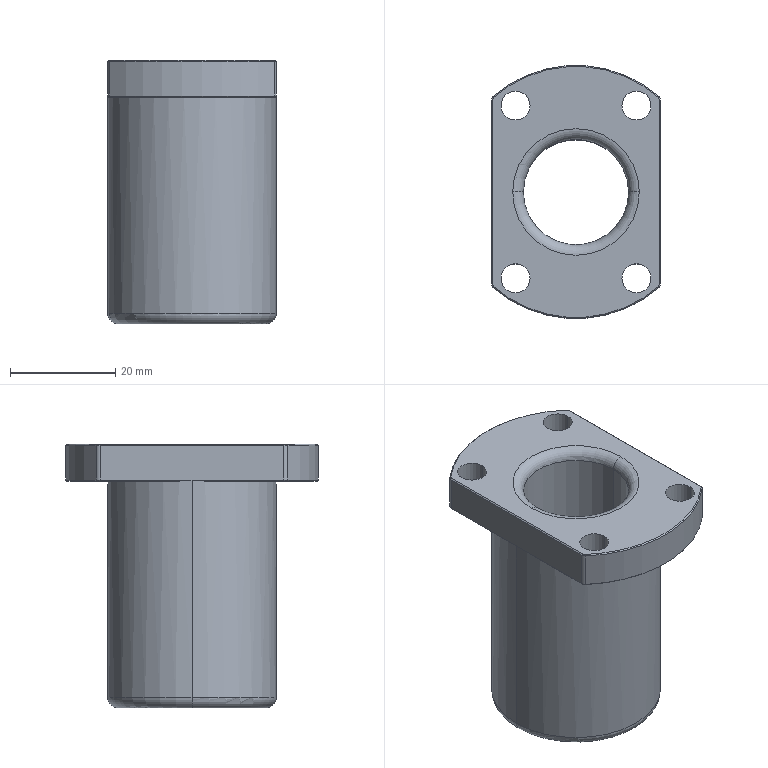Part | Creo | features DATUM PLANE 3, ROUND 3, CURVE 2, PROTRUSION 2, CHAMFER 1, COORDINATE SYSTEM 1 | 1 solid | 48 faces | box 32 x 48 x 50 mm | volume 27898 mm3 | cylinder 18 | plane 12 | cone 12 | torus 6 | commonest cylinder face diameters 5.5 x8 2 x4 20 x2 32 x2 48 x2
STEP:
#1=CARTESIAN_POINT('',(0.,0.,0.));
#2=DIRECTION('',(0.,0.,1.));
#3=DIRECTION('',(1.,0.,0.));
#4=AXIS2_PLACEMENT_3D('',#1,#2,#3);
#5=CARTESIAN_POINT('',(15.8,-2.522,0.));
#6=VERTEX_POINT('',#5);
#7=CARTESIAN_POINT('',(15.8,-17.436,-0.000000006));
#8=VERTEX_POINT('',#7);
#9=CARTESIAN_POINT('',(15.8,-2.522,0.));
#10=DIRECTION('',(0.,-1.,0.));
#11=VECTOR('',#10,14.914);
#12=LINE('',#9,#11);
#13=EDGE_CURVE('',#6,#8,#12,.T.);
#14=ORIENTED_EDGE('',*,*,#13,.F.);
#15=CARTESIAN_POINT('',(-15.8,-2.522,0.));
#16=VERTEX_POINT('',#15);
#17=CARTESIAN_POINT('',(0.,0.,0.));
#18=DIRECTION('',(0.,0.,-1.));
#19=DIRECTION('',(0.9875,-0.1576,0.));
#20=AXIS2_PLACEMENT_3D('',#17,#18,#19);
#21=CIRCLE('',#20,16.);
#22=EDGE_CURVE('',#6,#16,#21,.T.);
#23=ORIENTED_EDGE('',*,*,#22,.T.);
#24=CARTESIAN_POINT('',(-15.8,-17.436,0.));
#25=VERTEX_POINT('',#24);
#26=CARTESIAN_POINT('',(-15.8,-17.436,-0.000000002));
#27=DIRECTION('',(0.,1.,0.));
#28=VECTOR('',#27,14.914);
#29=LINE('',#26,#28);
#30=EDGE_CURVE('',#25,#16,#29,.T.);
#31=ORIENTED_EDGE('',*,*,#30,.F.);
#32=CARTESIAN_POINT('',(-15.522,-18.042,0.));
#33=VERTEX_POINT('',#32);
#34=CARTESIAN_POINT('',(-15.,-17.436,0.));
#35=DIRECTION('',(0.,0.,-1.));
#36=DIRECTION('',(-0.6522,-0.7581,0.));
#37=AXIS2_PLACEMENT_3D('',#34,#35,#36);
#38=CIRCLE('',#37,0.8);
#39=EDGE_CURVE('',#33,#25,#38,.T.);
#40=ORIENTED_EDGE('',*,*,#39,.F.);
#41=CARTESIAN_POINT('',(15.522,-18.042,0.));
#42=VERTEX_POINT('',#41);
#43=CARTESIAN_POINT('',(0.,0.,0.));
#44=DIRECTION('',(0.,0.,-1.));
#45=DIRECTION('',(0.6522,-0.7581,0.));
#46=AXIS2_PLACEMENT_3D('',#43,#44,#45);
#47=CIRCLE('',#46,23.8);
#48=EDGE_CURVE('',#42,#33,#47,.T.);
#49=ORIENTED_EDGE('',*,*,#48,.F.);
#50=CARTESIAN_POINT('',(15.,-17.436,0.));
#51=DIRECTION('',(0.,0.,-1.));
#52=DIRECTION('',(1.,0.,0.));
#53=AXIS2_PLACEMENT_3D('',#50,#51,#52);
#54=CIRCLE('',#53,0.8);
#55=EDGE_CURVE('',#8,#42,#54,.T.);
#56=ORIENTED_EDGE('',*,*,#55,.F.);
#57=EDGE_LOOP('',(#14,#23,#31,#40,#49,#56));
#58=FACE_OUTER_BOUND('',#57,.F.);
#59=CARTESIAN_POINT('',(14.222,-16.38,0.));
#60=VERTEX_POINT('',#59);
#61=CARTESIAN_POINT('',(8.722,-16.38,0.));
#62=VERTEX_POINT('',#61);
#63=CARTESIAN_POINT('',(11.472,-16.38,0.));
#64=DIRECTION('',(0.,0.,-1.));
#65=DIRECTION('',(1.,0.,0.));
#66=AXIS2_PLACEMENT_3D('',#63,#64,#65);
#67=CIRCLE('',#66,2.75);
#68=EDGE_CURVE('',#60,#62,#67,.T.);
#69=ORIENTED_EDGE('',*,*,#68,.T.);
#70=CARTESIAN_POINT('',(11.472,-16.38,0.));
#71=DIRECTION('',(0.,0.,-1.));
#72=DIRECTION('',(-1.,0.,0.));
#73=AXIS2_PLACEMENT_3D('',#70,#71,#72);
#74=CIRCLE('',#73,2.75);
#75=EDGE_CURVE('',#62,#60,#74,.T.);
#76=ORIENTED_EDGE('',*,*,#75,.T.);
#77=EDGE_LOOP('',(#69,#76));
#78=FACE_BOUND('',#77,.F.);
#79=CARTESIAN_POINT('',(-8.722,-16.38,0.));
#80=VERTEX_POINT('',#79);
#81=CARTESIAN_POINT('',(-14.222,-16.38,0.));
#82=VERTEX_POINT('',#81);
#83=CARTESIAN_POINT('',(-11.472,-16.38,0.));
#84=DIRECTION('',(0.,0.,-1.));
#85=DIRECTION('',(1.,0.,0.));
#86=AXIS2_PLACEMENT_3D('',#83,#84,#85);
#87=CIRCLE('',#86,2.75);
#88=EDGE_CURVE('',#80,#82,#87,.T.);
#89=ORIENTED_EDGE('',*,*,#88,.T.);
#90=CARTESIAN_POINT('',(-11.472,-16.38,0.));
#91=DIRECTION('',(0.,0.,-1.));
#92=DIRECTION('',(-1.,0.,0.));
#93=AXIS2_PLACEMENT_3D('',#90,#91,#92);
#94=CIRCLE('',#93,2.75);
#95=EDGE_CURVE('',#82,#80,#94,.T.);
#96=ORIENTED_EDGE('',*,*,#95,.T.);
#97=EDGE_LOOP('',(#89,#96));
#98=FACE_BOUND('',#97,.F.);
#99=CARTESIAN_POINT('',(0.,0.,0.));
#100=DIRECTION('',(0.,0.,1.));
#101=DIRECTION('',(1.,0.,0.));
#102=AXIS2_PLACEMENT_3D('',#99,#100,#101);
#103=PLANE('',#102);
#104=ADVANCED_FACE('',(#58,#78,#98),#103,.F.);
#105=CARTESIAN_POINT('',(15.8,17.436,-0.000000002));
#106=VERTEX_POINT('',#105);
#107=CARTESIAN_POINT('',(15.8,2.522,0.));
#108=VERTEX_POINT('',#107);
#109=CARTESIAN_POINT('',(15.8,17.436,-0.000000002));
#110=DIRECTION('',(0.,-1.,0.));
#111=VECTOR('',#110,14.914);
#112=LINE('',#109,#111);
#113=EDGE_CURVE('',#106,#108,#112,.T.);
#114=ORIENTED_EDGE('',*,*,#113,.F.);
#115=CARTESIAN_POINT('',(15.522,18.042,0.));
#116=VERTEX_POINT('',#115);
#117=CARTESIAN_POINT('',(15.,17.436,0.));
#118=DIRECTION('',(0.,0.,-1.));
#119=DIRECTION('',(0.6522,0.7581,0.));
#120=AXIS2_PLACEMENT_3D('',#117,#118,#119);
#121=CIRCLE('',#120,0.8);
#122=EDGE_CURVE('',#116,#106,#121,.T.);
#123=ORIENTED_EDGE('',*,*,#122,.F.);
#124=CARTESIAN_POINT('',(-15.522,18.042,0.));
#125=VERTEX_POINT('',#124);
#126=CARTESIAN_POINT('',(0.,0.,0.));
#127=DIRECTION('',(0.,0.,-1.));
#128=DIRECTION('',(-0.6522,0.7581,0.));
#129=AXIS2_PLACEMENT_3D('',#126,#127,#128);
#130=CIRCLE('',#129,23.8);
#131=EDGE_CURVE('',#125,#116,#130,.T.);
#132=ORIENTED_EDGE('',*,*,#131,.F.);
#133=CARTESIAN_POINT('',(-15.8,17.436,0.));
#134=VERTEX_POINT('',#133);
#135=CARTESIAN_POINT('',(-15.,17.436,0.));
#136=DIRECTION('',(0.,0.,-1.));
#137=DIRECTION('',(-1.,0.,0.));
#138=AXIS2_PLACEMENT_3D('',#135,#136,#137);
#139=CIRCLE('',#138,0.8);
#140=EDGE_CURVE('',#134,#125,#139,.T.);
#141=ORIENTED_EDGE('',*,*,#140,.F.);
#142=CARTESIAN_POINT('',(-15.8,2.522,0.));
#143=VERTEX_POINT('',#142);
#144=CARTESIAN_POINT('',(-15.8,2.522,0.));
#145=DIRECTION('',(0.,1.,0.));
#146=VECTOR('',#145,14.914);
#147=LINE('',#144,#146);
#148=EDGE_CURVE('',#143,#134,#147,.T.);
#149=ORIENTED_EDGE('',*,*,#148,.F.);
#150=CARTESIAN_POINT('',(0.,0.,0.));
#151=DIRECTION('',(0.,0.,-1.));
#152=DIRECTION('',(-0.9875,0.1576,0.));
#153=AXIS2_PLACEMENT_3D('',#150,#151,#152);
#154=CIRCLE('',#153,16.);
#155=EDGE_CURVE('',#143,#108,#154,.T.);
#156=ORIENTED_EDGE('',*,*,#155,.T.);
#157=EDGE_LOOP('',(#114,#123,#132,#141,#149,#156));
#158=FACE_OUTER_BOUND('',#157,.F.);
#159=CARTESIAN_POINT('',(14.222,16.38,0.));
#160=VERTEX_POINT('',#159);
#161=CARTESIAN_POINT('',(8.722,16.38,0.));
#162=VERTEX_POINT('',#161);
#163=CARTESIAN_POINT('',(11.472,16.38,0.));
#164=DIRECTION('',(0.,0.,-1.));
#165=DIRECTION('',(1.,0.,0.));
#166=AXIS2_PLACEMENT_3D('',#163,#164,#165);
#167=CIRCLE('',#166,2.75);
#168=EDGE_CURVE('',#160,#162,#167,.T.);
#169=ORIENTED_EDGE('',*,*,#168,.T.);
#170=CARTESIAN_POINT('',(11.472,16.38,0.));
#171=DIRECTION('',(0.,0.,-1.));
#172=DIRECTION('',(-1.,0.,0.));
#173=AXIS2_PLACEMENT_3D('',#170,#171,#172);
#174=CIRCLE('',#173,2.75);
#175=EDGE_CURVE('',#162,#160,#174,.T.);
#176=ORIENTED_EDGE('',*,*,#175,.T.);
#177=EDGE_LOOP('',(#169,#176));
#178=FACE_BOUND('',#177,.F.);
#179=CARTESIAN_POINT('',(-8.722,16.38,0.));
#180=VERTEX_POINT('',#179);
#181=CARTESIAN_POINT('',(-14.222,16.38,0.));
#182=VERTEX_POINT('',#181);
#183=CARTESIAN_POINT('',(-11.472,16.38,0.));
#184=DIRECTION('',(0.,0.,-1.));
#185=DIRECTION('',(1.,0.,0.));
#186=AXIS2_PLACEMENT_3D('',#183,#184,#185);
#187=CIRCLE('',#186,2.75);
#188=EDGE_CURVE('',#180,#182,#187,.T.);
#189=ORIENTED_EDGE('',*,*,#188,.T.);
#190=CARTESIAN_POINT('',(-11.472,16.38,0.));
#191=DIRECTION('',(0.,0.,-1.));
#192=DIRECTION('',(-1.,0.,0.));
#193=AXIS2_PLACEMENT_3D('',#190,#191,#192);
#194=CIRCLE('',#193,2.75);
#195=EDGE_CURVE('',#182,#180,#194,.T.);
#196=ORIENTED_EDGE('',*,*,#195,.T.);
#197=EDGE_LOOP('',(#189,#196));
#198=FACE_BOUND('',#197,.F.);
#199=CARTESIAN_POINT('',(0.,0.,0.));
#200=DIRECTION('',(0.,0.,1.));
#201=DIRECTION('',(1.,0.,0.));
#202=AXIS2_PLACEMENT_3D('',#199,#200,#201);
#203=PLANE('',#202);
#204=ADVANCED_FACE('',(#158,#178,#198),#203,.F.);
#205=ORIENTED_EDGE('',*,*,#168,.F.);
#206=CARTESIAN_POINT('',(14.222,16.38,7.));
#207=VERTEX_POINT('',#206);
#208=CARTESIAN_POINT('',(14.222,16.38,0.));
#209=DIRECTION('',(0.,0.,1.));
#210=VECTOR('',#209,7.);
#211=LINE('',#208,#210);
#212=EDGE_CURVE('',#160,#207,#211,.T.);
#213=ORIENTED_EDGE('',*,*,#212,.T.);
#214=CARTESIAN_POINT('',(8.722,16.38,7.));
#215=VERTEX_POINT('',#214);
#216=CARTESIAN_POINT('',(11.472,16.38,7.));
#217=DIRECTION('',(0.,0.,-1.));
#218=DIRECTION('',(1.,0.,0.));
#219=AXIS2_PLACEMENT_3D('',#216,#217,#218);
#220=CIRCLE('',#219,2.75);
#221=EDGE_CURVE('',#207,#215,#220,.T.);
#222=ORIENTED_EDGE('',*,*,#221,.T.);
#223=CARTESIAN_POINT('',(8.722,16.38,0.));
#224=DIRECTION('',(0.,0.,1.));
#225=VECTOR('',#224,7.);
#226=LINE('',#223,#225);
#227=EDGE_CURVE('',#162,#215,#226,.T.);
#228=ORIENTED_EDGE('',*,*,#227,.F.);
#229=EDGE_LOOP('',(#205,#213,#222,#228));
#230=FACE_OUTER_BOUND('',#229,.F.);
#231=CARTESIAN_POINT('',(11.472,16.38,0.));
#232=DIRECTION('',(0.,0.,1.));
#233=DIRECTION('',(1.,0.,0.));
#234=AXIS2_PLACEMENT_3D('',#231,#232,#233);
#235=CYLINDRICAL_SURFACE('',#234,2.75);
#236=ADVANCED_FACE('',(#230),#235,.F.);
#237=ORIENTED_EDGE('',*,*,#175,.F.);
#238=ORIENTED_EDGE('',*,*,#227,.T.);
#239=CARTESIAN_POINT('',(11.472,16.38,7.));
#240=DIRECTION('',(0.,0.,-1.));
#241=DIRECTION('',(-1.,0.,0.));
#242=AXIS2_PLACEMENT_3D('',#239,#240,#241);
#243=CIRCLE('',#242,2.75);
#244=EDGE_CURVE('',#215,#207,#243,.T.);
#245=ORIENTED_EDGE('',*,*,#244,.T.);
#246=ORIENTED_EDGE('',*,*,#212,.F.);
#247=EDGE_LOOP('',(#237,#238,#245,#246));
#248=FACE_OUTER_BOUND('',#247,.F.);
#249=CARTESIAN_POINT('',(11.472,16.38,0.));
#250=DIRECTION('',(0.,0.,1.));
#251=DIRECTION('',(1.,0.,0.));
#252=AXIS2_PLACEMENT_3D('',#249,#250,#251);
#253=CYLINDRICAL_SURFACE('',#252,2.75);
#254=ADVANCED_FACE('',(#248),#253,.F.);
#255=CARTESIAN_POINT('',(-15.8,-17.436,7.));
#256=VERTEX_POINT('',#255);
#257=CARTESIAN_POINT('',(-15.522,-18.042,7.));
#258=VERTEX_POINT('',#257);
#259=CARTESIAN_POINT('',(-15.,-17.436,7.));
#260=DIRECTION('',(0.,0.,1.));
#261=DIRECTION('',(-1.,0.,0.));
#262=AXIS2_PLACEMENT_3D('',#259,#260,#261);
#263=CIRCLE('',#262,0.8);
#264=EDGE_CURVE('',#256,#258,#263,.T.);
#265=ORIENTED_EDGE('',*,*,#264,.F.);
#266=CARTESIAN_POINT('',(-15.8,17.436,7.));
#267=VERTEX_POINT('',#266);
#268=CARTESIAN_POINT('',(-15.8,17.436,7.));
#269=DIRECTION('',(0.,-1.,0.));
#270=VECTOR('',#269,34.871);
#271=LINE('',#268,#270);
#272=EDGE_CURVE('',#267,#256,#271,.T.);
#273=ORIENTED_EDGE('',*,*,#272,.F.);
#274=CARTESIAN_POINT('',(-15.522,18.042,7.));
#275=VERTEX_POINT('',#274);
#276=CARTESIAN_POINT('',(-15.,17.436,7.));
#277=DIRECTION('',(0.,0.,1.));
#278=DIRECTION('',(-0.6522,0.7581,0.));
#279=AXIS2_PLACEMENT_3D('',#276,#277,#278);
#280=CIRCLE('',#279,0.8);
#281=EDGE_CURVE('',#275,#267,#280,.T.);
#282=ORIENTED_EDGE('',*,*,#281,.F.);
#283=CARTESIAN_POINT('',(15.522,18.042,7.));
#284=VERTEX_POINT('',#283);
#285=CARTESIAN_POINT('',(0.,0.,7.));
#286=DIRECTION('',(0.,0.,1.));
#287=DIRECTION('',(0.6522,0.7581,0.));
#288=AXIS2_PLACEMENT_3D('',#285,#286,#287);
#289=CIRCLE('',#288,23.8);
#290=EDGE_CURVE('',#284,#275,#289,.T.);
#291=ORIENTED_EDGE('',*,*,#290,.F.);
#292=CARTESIAN_POINT('',(15.8,17.436,7.));
#293=VERTEX_POINT('',#292);
#294=CARTESIAN_POINT('',(15.,17.436,7.));
#295=DIRECTION('',(0.,0.,1.));
#296=DIRECTION('',(1.,0.,0.));
#297=AXIS2_PLACEMENT_3D('',#294,#295,#296);
#298=CIRCLE('',#297,0.8);
#299=EDGE_CURVE('',#293,#284,#298,.T.);
#300=ORIENTED_EDGE('',*,*,#299,.F.);
#301=CARTESIAN_POINT('',(15.8,-17.436,7.));
#302=VERTEX_POINT('',#301);
#303=CARTESIAN_POINT('',(15.8,-17.436,7.));
#304=DIRECTION('',(0.,1.,0.));
#305=VECTOR('',#304,34.871);
#306=LINE('',#303,#305);
#307=EDGE_CURVE('',#302,#293,#306,.T.);
#308=ORIENTED_EDGE('',*,*,#307,.F.);
#309=CARTESIAN_POINT('',(15.522,-18.042,7.));
#310=VERTEX_POINT('',#309);
#311=CARTESIAN_POINT('',(15.,-17.436,7.));
#312=DIRECTION('',(0.,0.,1.));
#313=DIRECTION('',(0.6522,-0.7581,0.));
#314=AXIS2_PLACEMENT_3D('',#311,#312,#313);
#315=CIRCLE('',#314,0.8);
#316=EDGE_CURVE('',#310,#302,#315,.T.);
#317=ORIENTED_EDGE('',*,*,#316,.F.);
#318=CARTESIAN_POINT('',(0.,0.,7.));
#319=DIRECTION('',(0.,0.,1.));
#320=DIRECTION('',(-0.6522,-0.7581,0.));
#321=AXIS2_PLACEMENT_3D('',#318,#319,#320);
#322=CIRCLE('',#321,23.8);
#323=EDGE_CURVE('',#258,#310,#322,.T.);
#324=ORIENTED_EDGE('',*,*,#323,.F.);
#325=EDGE_LOOP('',(#265,#273,#282,#291,#300,#308,#317,#324));
#326=FACE_OUTER_BOUND('',#325,.F.);
#327=CARTESIAN_POINT('',(-8.722,16.38,7.));
#328=VERTEX_POINT('',#327);
#329=CARTESIAN_POINT('',(-14.222,16.38,7.));
#330=VERTEX_POINT('',#329);
#331=CARTESIAN_POINT('',(-11.472,16.38,7.));
#332=DIRECTION('',(0.,0.,-1.));
#333=DIRECTION('',(1.,0.,0.));
#334=AXIS2_PLACEMENT_3D('',#331,#332,#333);
#335=CIRCLE('',#334,2.75);
#336=EDGE_CURVE('',#328,#330,#335,.T.);
#337=ORIENTED_EDGE('',*,*,#336,.F.);
#338=CARTESIAN_POINT('',(-11.472,16.38,7.));
#339=DIRECTION('',(0.,0.,-1.));
#340=DIRECTION('',(-1.,0.,0.));
#341=AXIS2_PLACEMENT_3D('',#338,#339,#340);
#342=CIRCLE('',#341,2.75);
#343=EDGE_CURVE('',#330,#328,#342,.T.);
#344=ORIENTED_EDGE('',*,*,#343,.F.);
#345=EDGE_LOOP('',(#337,#344));
#346=FACE_BOUND('',#345,.F.);
#347=CARTESIAN_POINT('',(14.222,-16.38,7.));
#348=VERTEX_POINT('',#347);
#349=CARTESIAN_POINT('',(8.722,-16.38,7.));
#350=VERTEX_POINT('',#349);
#351=CARTESIAN_POINT('',(11.472,-16.38,7.));
#352=DIRECTION('',(0.,0.,-1.));
#353=DIRECTION('',(1.,0.,0.));
#354=AXIS2_PLACEMENT_3D('',#351,#352,#353);
#355=CIRCLE('',#354,2.75);
#356=EDGE_CURVE('',#348,#350,#355,.T.);
#357=ORIENTED_EDGE('',*,*,#356,.F.);
#358=CARTESIAN_POINT('',(11.472,-16.38,7.));
#359=DIRECTION('',(0.,0.,-1.));
#360=DIRECTION('',(-1.,0.,0.));
#361=AXIS2_PLACEMENT_3D('',#358,#359,#360);
#362=CIRCLE('',#361,2.75);
#363=EDGE_CURVE('',#350,#348,#362,.T.);
#364=ORIENTED_EDGE('',*,*,#363,.F.);
#365=EDGE_LOOP('',(#357,#364));
#366=FACE_BOUND('',#365,.F.);
#367=CARTESIAN_POINT('',(-8.722,-16.38,7.));
#368=VERTEX_POINT('',#367);
#369=CARTESIAN_POINT('',(-14.222,-16.38,7.));
#370=VERTEX_POINT('',#369);
#371=CARTESIAN_POINT('',(-11.472,-16.38,7.));
#372=DIRECTION('',(0.,0.,-1.));
#373=DIRECTION('',(1.,0.,0.));
#374=AXIS2_PLACEMENT_3D('',#371,#372,#373);
#375=CIRCLE('',#374,2.75);
#376=EDGE_CURVE('',#368,#370,#375,.T.);
#377=ORIENTED_EDGE('',*,*,#376,.F.);
#378=CARTESIAN_POINT('',(-11.472,-16.38,7.));
#379=DIRECTION('',(0.,0.,-1.));
#380=DIRECTION('',(-1.,0.,0.));
#381=AXIS2_PLACEMENT_3D('',#378,#379,#380);
#382=CIRCLE('',#381,2.75);
#383=EDGE_CURVE('',#370,#368,#382,.T.);
#384=ORIENTED_EDGE('',*,*,#383,.F.);
#385=EDGE_LOOP('',(#377,#384));
#386=FACE_BOUND('',#385,.F.);
#387=ORIENTED_EDGE('',*,*,#221,.F.);
#388=ORIENTED_EDGE('',*,*,#244,.F.);
#389=EDGE_LOOP('',(#387,#388));
#390=FACE_BOUND('',#389,.F.);
#391=CARTESIAN_POINT('',(-12.,0.,7.));
#392=VERTEX_POINT('',#391);
#393=CARTESIAN_POINT('',(12.,0.,7.));
#394=VERTEX_POINT('',#393);
#395=CARTESIAN_POINT('',(0.,0.,7.));
#396=DIRECTION('',(0.,0.,-1.));
#397=DIRECTION('',(-1.,0.,0.));
#398=AXIS2_PLACEMENT_3D('',#395,#396,#397);
#399=CIRCLE('',#398,12.);
#400=EDGE_CURVE('',#392,#394,#399,.T.);
#401=ORIENTED_EDGE('',*,*,#400,.F.);
#402=CARTESIAN_POINT('',(0.,0.,7.));
#403=DIRECTION('',(0.,0.,-1.));
#404=DIRECTION('',(1.,0.,0.));
#405=AXIS2_PLACEMENT_3D('',#402,#403,#404);
#406=CIRCLE('',#405,12.);
#407=EDGE_CURVE('',#394,#392,#406,.T.);
#408=ORIENTED_EDGE('',*,*,#407,.F.);
#409=EDGE_LOOP('',(#401,#408));
#410=FACE_BOUND('',#409,.F.);
#411=CARTESIAN_POINT('',(0.,0.,7.));
#412=DIRECTION('',(0.,0.,1.));
#413=DIRECTION('',(1.,0.,0.));
#414=AXIS2_PLACEMENT_3D('',#411,#412,#413);
#415=PLANE('',#414);
#416=ADVANCED_FACE('',(#326,#346,#366,#386,#390,#410),#415,.T.);
#417=ORIENTED_EDGE('',*,*,#188,.F.);
#418=CARTESIAN_POINT('',(-8.722,16.38,0.));
#419=DIRECTION('',(0.,0.,1.));
#420=VECTOR('',#419,7.);
#421=LINE('',#418,#420);
#422=EDGE_CURVE('',#180,#328,#421,.T.);
#423=ORIENTED_EDGE('',*,*,#422,.T.);
#424=ORIENTED_EDGE('',*,*,#336,.T.);
#425=CARTESIAN_POINT('',(-14.222,16.38,0.));
#426=DIRECTION('',(0.,0.,1.));
#427=VECTOR('',#426,7.);
#428=LINE('',#425,#427);
#429=EDGE_CURVE('',#182,#330,#428,.T.);
#430=ORIENTED_EDGE('',*,*,#429,.F.);
#431=EDGE_LOOP('',(#417,#423,#424,#430));
#432=FACE_OUTER_BOUND('',#431,.F.);
#433=CARTESIAN_POINT('',(-11.472,16.38,0.));
#434=DIRECTION('',(0.,0.,1.));
#435=DIRECTION('',(1.,0.,0.));
#436=AXIS2_PLACEMENT_3D('',#433,#434,#435);
#437=CYLINDRICAL_SURFACE('',#436,2.75);
#438=ADVANCED_FACE('',(#432),#437,.F.);
#439=ORIENTED_EDGE('',*,*,#195,.F.);
#440=ORIENTED_EDGE('',*,*,#429,.T.);
#441=ORIENTED_EDGE('',*,*,#343,.T.);
#442=ORIENTED_EDGE('',*,*,#422,.F.);
#443=EDGE_LOOP('',(#439,#440,#441,#442));
#444=FACE_OUTER_BOUND('',#443,.F.);
#445=CARTESIAN_POINT('',(-11.472,16.38,0.));
#446=DIRECTION('',(0.,0.,1.));
#447=DIRECTION('',(1.,0.,0.));
#448=AXIS2_PLACEMENT_3D('',#445,#446,#447);
#449=CYLINDRICAL_SURFACE('',#448,2.75);
#450=ADVANCED_FACE('',(#444),#449,.F.);
#451=ORIENTED_EDGE('',*,*,#68,.F.);
#452=CARTESIAN_POINT('',(14.222,-16.38,0.));
#453=DIRECTION('',(0.,0.,1.));
#454=VECTOR('',#453,7.);
#455=LINE('',#452,#454);
#456=EDGE_CURVE('',#60,#348,#455,.T.);
#457=ORIENTED_EDGE('',*,*,#456,.T.);
#458=ORIENTED_EDGE('',*,*,#356,.T.);
#459=CARTESIAN_POINT('',(8.722,-16.38,0.));
#460=DIRECTION('',(0.,0.,1.));
#461=VECTOR('',#460,7.);
#462=LINE('',#459,#461);
#463=EDGE_CURVE('',#62,#350,#462,.T.);
#464=ORIENTED_EDGE('',*,*,#463,.F.);
#465=EDGE_LOOP('',(#451,#457,#458,#464));
#466=FACE_OUTER_BOUND('',#465,.F.);
#467=CARTESIAN_POINT('',(11.472,-16.38,0.));
#468=DIRECTION('',(0.,0.,1.));
#469=DIRECTION('',(1.,0.,0.));
#470=AXIS2_PLACEMENT_3D('',#467,#468,#469);
#471=CYLINDRICAL_SURFACE('',#470,2.75);
#472=ADVANCED_FACE('',(#466),#471,.F.);
#473=ORIENTED_EDGE('',*,*,#75,.F.);
#474=ORIENTED_EDGE('',*,*,#463,.T.);
#475=ORIENTED_EDGE('',*,*,#363,.T.);
#476=ORIENTED_EDGE('',*,*,#456,.F.);
#477=EDGE_LOOP('',(#473,#474,#475,#476));
#478=FACE_OUTER_BOUND('',#477,.F.);
#479=CARTESIAN_POINT('',(11.472,-16.38,0.));
#480=DIRECTION('',(0.,0.,1.));
#481=DIRECTION('',(1.,0.,0.));
#482=AXIS2_PLACEMENT_3D('',#479,#480,#481);
#483=CYLINDRICAL_SURFACE('',#482,2.75);
#484=ADVANCED_FACE('',(#478),#483,.F.);
#485=ORIENTED_EDGE('',*,*,#88,.F.);
#486=CARTESIAN_POINT('',(-8.722,-16.38,0.));
#487=DIRECTION('',(0.,0.,1.));
#488=VECTOR('',#487,7.);
#489=LINE('',#486,#488);
#490=EDGE_CURVE('',#80,#368,#489,.T.);
#491=ORIENTED_EDGE('',*,*,#490,.T.);
#492=ORIENTED_EDGE('',*,*,#376,.T.);
#493=CARTESIAN_POINT('',(-14.222,-16.38,0.));
#494=DIRECTION('',(0.,0.,1.));
#495=VECTOR('',#494,7.);
#496=LINE('',#493,#495);
#497=EDGE_CURVE('',#82,#370,#496,.T.);
#498=ORIENTED_EDGE('',*,*,#497,.F.);
#499=EDGE_LOOP('',(#485,#491,#492,#498));
#500=FACE_OUTER_BOUND('',#499,.F.);
#501=CARTESIAN_POINT('',(-11.472,-16.38,0.));
#502=DIRECTION('',(0.,0.,1.));
#503=DIRECTION('',(1.,0.,0.));
#504=AXIS2_PLACEMENT_3D('',#501,#502,#503);
#505=CYLINDRICAL_SURFACE('',#504,2.75);
#506=ADVANCED_FACE('',(#500),#505,.F.);
#507=ORIENTED_EDGE('',*,*,#95,.F.);
#508=ORIENTED_EDGE('',*,*,#497,.T.);
#509=ORIENTED_EDGE('',*,*,#383,.T.);
#510=ORIENTED_EDGE('',*,*,#490,.F.);
#511=EDGE_LOOP('',(#507,#508,#509,#510));
#512=FACE_OUTER_BOUND('',#511,.F.);
#513=CARTESIAN_POINT('',(-11.472,-16.38,0.));
#514=DIRECTION('',(0.,0.,1.));
#515=DIRECTION('',(1.,0.,0.));
#516=AXIS2_PLACEMENT_3D('',#513,#514,#515);
#517=CYLINDRICAL_SURFACE('',#516,2.75);
#518=ADVANCED_FACE('',(#512),#517,.F.);
#519=ORIENTED_EDGE('',*,*,#264,.T.);
#520=CARTESIAN_POINT('',(-15.652,-18.194,6.8));
#521=VERTEX_POINT('',#520);
#522=CARTESIAN_POINT('',(-15.522,-18.042,7.));
#523=DIRECTION('',(-0.4612,-0.536,-0.7071));
#524=VECTOR('',#523,0.2828);
#525=LINE('',#522,#524);
#526=EDGE_CURVE('',#258,#521,#525,.T.);
#527=ORIENTED_EDGE('',*,*,#526,.T.);
#528=CARTESIAN_POINT('',(-16.,-17.436,6.8));
#529=VERTEX_POINT('',#528);
#530=CARTESIAN_POINT('',(-15.,-17.436,6.8));
#531=DIRECTION('',(0.,0.,1.));
#532=DIRECTION('',(-1.,0.,0.));
#533=AXIS2_PLACEMENT_3D('',#530,#531,#532);
#534=CIRCLE('',#533,1.);
#535=EDGE_CURVE('',#529,#521,#534,.T.);
#536=ORIENTED_EDGE('',*,*,#535,.F.);
#537=CARTESIAN_POINT('',(-15.8,-17.436,7.));
#538=DIRECTION('',(-0.7071,0.000000006,-0.7071));
#539=VECTOR('',#538,0.2828);
#540=LINE('',#537,#539);
#541=EDGE_CURVE('',#256,#529,#540,.T.);
#542=ORIENTED_EDGE('',*,*,#541,.F.);
#543=EDGE_LOOP('',(#519,#527,#536,#542));
#544=FACE_OUTER_BOUND('',#543,.F.);
#545=CARTESIAN_POINT('',(-15.,-17.436,6.9));
#546=DIRECTION('',(0.,0.,-1.));
#547=DIRECTION('',(0.,-1.,0.));
#548=AXIS2_PLACEMENT_3D('',#545,#546,#547);
#549=CONICAL_SURFACE('',#548,0.9,45.);
#550=ADVANCED_FACE('',(#544),#549,.T.);
#551=ORIENTED_EDGE('',*,*,#323,.T.);
#552=CARTESIAN_POINT('',(15.652,-18.194,6.8));
#553=VERTEX_POINT('',#552);
#554=CARTESIAN_POINT('',(15.522,-18.042,7.));
#555=DIRECTION('',(0.4612,-0.536,-0.7071));
#556=VECTOR('',#555,0.2828);
#557=LINE('',#554,#556);
#558=EDGE_CURVE('',#310,#553,#557,.T.);
#559=ORIENTED_EDGE('',*,*,#558,.T.);
#560=CARTESIAN_POINT('',(0.,0.,6.8));
#561=DIRECTION('',(0.,0.,1.));
#562=DIRECTION('',(-0.6522,-0.7581,0.));
#563=AXIS2_PLACEMENT_3D('',#560,#561,#562);
#564=CIRCLE('',#563,24.);
#565=EDGE_CURVE('',#521,#553,#564,.T.);
#566=ORIENTED_EDGE('',*,*,#565,.F.);
#567=ORIENTED_EDGE('',*,*,#526,.F.);
#568=EDGE_LOOP('',(#551,#559,#566,#567));
#569=FACE_OUTER_BOUND('',#568,.F.);
#570=CARTESIAN_POINT('',(0.,0.,6.9));
#571=DIRECTION('',(0.,0.,-1.));
#572=DIRECTION('',(0.,-1.,0.));
#573=AXIS2_PLACEMENT_3D('',#570,#571,#572);
#574=CONICAL_SURFACE('',#573,23.9,45.);
#575=ADVANCED_FACE('',(#569),#574,.T.);
#576=ORIENTED_EDGE('',*,*,#316,.T.);
#577=CARTESIAN_POINT('',(16.,-17.436,6.8));
#578=VERTEX_POINT('',#577);
#579=CARTESIAN_POINT('',(15.8,-17.436,7.));
#580=DIRECTION('',(0.7071,0.000000005,-0.7071));
#581=VECTOR('',#580,0.2828);
#582=LINE('',#579,#581);
#583=EDGE_CURVE('',#302,#578,#582,.T.);
#584=ORIENTED_EDGE('',*,*,#583,.T.);
#585=CARTESIAN_POINT('',(15.,-17.436,6.8));
#586=DIRECTION('',(0.,0.,1.));
#587=DIRECTION('',(0.6522,-0.7581,0.));
#588=AXIS2_PLACEMENT_3D('',#585,#586,#587);
#589=CIRCLE('',#588,1.);
#590=EDGE_CURVE('',#553,#578,#589,.T.);
#591=ORIENTED_EDGE('',*,*,#590,.F.);
#592=ORIENTED_EDGE('',*,*,#558,.F.);
#593=EDGE_LOOP('',(#576,#584,#591,#592));
#594=FACE_OUTER_BOUND('',#593,.F.);
#595=CARTESIAN_POINT('',(15.,-17.436,6.9));
#596=DIRECTION('',(0.,0.,-1.));
#597=DIRECTION('',(0.,-1.,0.));
#598=AXIS2_PLACEMENT_3D('',#595,#596,#597);
#599=CONICAL_SURFACE('',#598,0.9,45.);
#600=ADVANCED_FACE('',(#594),#599,.T.);
#601=ORIENTED_EDGE('',*,*,#307,.T.);
#602=CARTESIAN_POINT('',(16.,17.436,6.8));
#603=VERTEX_POINT('',#602);
#604=CARTESIAN_POINT('',(15.8,17.436,7.));
#605=DIRECTION('',(0.7071,-0.000000006,-0.7071));
#606=VECTOR('',#605,0.2828);
#607=LINE('',#604,#606);
#608=EDGE_CURVE('',#293,#603,#607,.T.);
#609=ORIENTED_EDGE('',*,*,#608,.T.);
#610=CARTESIAN_POINT('',(16.,-17.436,6.8));
#611=DIRECTION('',(0.,1.,0.));
#612=VECTOR('',#611,34.871);
#613=LINE('',#610,#612);
#614=EDGE_CURVE('',#578,#603,#613,.T.);
#615=ORIENTED_EDGE('',*,*,#614,.F.);
#616=ORIENTED_EDGE('',*,*,#583,.F.);
#617=EDGE_LOOP('',(#601,#609,#615,#616));
#618=FACE_OUTER_BOUND('',#617,.F.);
#619=CARTESIAN_POINT('',(15.9,0.,6.9));
#620=DIRECTION('',(0.7071,0.,0.7071));
#621=DIRECTION('',(0.7071,0.,-0.7071));
#622=AXIS2_PLACEMENT_3D('',#619,#620,#621);
#623=PLANE('',#622);
#624=ADVANCED_FACE('',(#618),#623,.T.);
#625=ORIENTED_EDGE('',*,*,#299,.T.);
#626=CARTESIAN_POINT('',(15.652,18.194,6.8));
#627=VERTEX_POINT('',#626);
#628=CARTESIAN_POINT('',(15.522,18.042,7.));
#629=DIRECTION('',(0.4612,0.536,-0.7071));
#630=VECTOR('',#629,0.2828);
#631=LINE('',#628,#630);
#632=EDGE_CURVE('',#284,#627,#631,.T.);
#633=ORIENTED_EDGE('',*,*,#632,.T.);
#634=CARTESIAN_POINT('',(15.,17.436,6.8));
#635=DIRECTION('',(0.,0.,1.));
#636=DIRECTION('',(1.,0.,0.));
#637=AXIS2_PLACEMENT_3D('',#634,#635,#636);
#638=CIRCLE('',#637,1.);
#639=EDGE_CURVE('',#603,#627,#638,.T.);
#640=ORIENTED_EDGE('',*,*,#639,.F.);
#641=ORIENTED_EDGE('',*,*,#608,.F.);
#642=EDGE_LOOP('',(#625,#633,#640,#641));
#643=FACE_OUTER_BOUND('',#642,.F.);
#644=CARTESIAN_POINT('',(15.,17.436,6.9));
#645=DIRECTION('',(0.,0.,-1.));
#646=DIRECTION('',(0.,-1.,0.));
#647=AXIS2_PLACEMENT_3D('',#644,#645,#646);
#648=CONICAL_SURFACE('',#647,0.9,45.);
#649=ADVANCED_FACE('',(#643),#648,.T.);
#650=ORIENTED_EDGE('',*,*,#290,.T.);
#651=CARTESIAN_POINT('',(-15.652,18.194,6.8));
#652=VERTEX_POINT('',#651);
#653=CARTESIAN_POINT('',(-15.522,18.042,7.));
#654=DIRECTION('',(-0.4612,0.536,-0.7071));
#655=VECTOR('',#654,0.2828);
#656=LINE('',#653,#655);
#657=EDGE_CURVE('',#275,#652,#656,.T.);
#658=ORIENTED_EDGE('',*,*,#657,.T.);
#659=CARTESIAN_POINT('',(0.,0.,6.8));
#660=DIRECTION('',(0.,0.,1.));
#661=DIRECTION('',(0.6522,0.7581,0.));
#662=AXIS2_PLACEMENT_3D('',#659,#660,#661);
#663=CIRCLE('',#662,24.);
#664=EDGE_CURVE('',#627,#652,#663,.T.);
#665=ORIENTED_EDGE('',*,*,#664,.F.);
#666=ORIENTED_EDGE('',*,*,#632,.F.);
#667=EDGE_LOOP('',(#650,#658,#665,#666));
#668=FACE_OUTER_BOUND('',#667,.F.);
#669=CARTESIAN_POINT('',(0.,0.,6.9));
#670=DIRECTION('',(0.,0.,-1.));
#671=DIRECTION('',(0.,-1.,0.));
#672=AXIS2_PLACEMENT_3D('',#669,#670,#671);
#673=CONICAL_SURFACE('',#672,23.9,45.);
#674=ADVANCED_FACE('',(#668),#673,.T.);
#675=ORIENTED_EDGE('',*,*,#281,.T.);
#676=CARTESIAN_POINT('',(-16.,17.436,6.8));
#677=VERTEX_POINT('',#676);
#678=CARTESIAN_POINT('',(-15.8,17.436,7.));
#679=DIRECTION('',(-0.7071,-0.000000005,-0.7071));
#680=VECTOR('',#679,0.2828);
#681=LINE('',#678,#680);
#682=EDGE_CURVE('',#267,#677,#681,.T.);
#683=ORIENTED_EDGE('',*,*,#682,.T.);
#684=CARTESIAN_POINT('',(-15.,17.436,6.8));
#685=DIRECTION('',(0.,0.,1.));
#686=DIRECTION('',(-0.6522,0.7581,0.));
#687=AXIS2_PLACEMENT_3D('',#684,#685,#686);
#688=CIRCLE('',#687,1.);
#689=EDGE_CURVE('',#652,#677,#688,.T.);
#690=ORIENTED_EDGE('',*,*,#689,.F.);
#691=ORIENTED_EDGE('',*,*,#657,.F.);
#692=EDGE_LOOP('',(#675,#683,#690,#691));
#693=FACE_OUTER_BOUND('',#692,.F.);
#694=CARTESIAN_POINT('',(-15.,17.436,6.9));
#695=DIRECTION('',(0.,0.,-1.));
#696=DIRECTION('',(0.,-1.,0.));
#697=AXIS2_PLACEMENT_3D('',#694,#695,#696);
#698=CONICAL_SURFACE('',#697,0.9,45.);
#699=ADVANCED_FACE('',(#693),#698,.T.);
#700=ORIENTED_EDGE('',*,*,#272,.T.);
#701=ORIENTED_EDGE('',*,*,#541,.T.);
#702=CARTESIAN_POINT('',(-16.,17.436,6.8));
#703=DIRECTION('',(0.,-1.,0.));
#704=VECTOR('',#703,34.871);
#705=LINE('',#702,#704);
#706=EDGE_CURVE('',#677,#529,#705,.T.);
#707=ORIENTED_EDGE('',*,*,#706,.F.);
#708=ORIENTED_EDGE('',*,*,#682,.F.);
#709=EDGE_LOOP('',(#700,#701,#707,#708));
#710=FACE_OUTER_BOUND('',#709,.F.);
#711=CARTESIAN_POINT('',(-15.9,0.,6.9));
#712=DIRECTION('',(-0.7071,0.,0.7071));
#713=DIRECTION('',(-0.7071,0.,-0.7071));
#714=AXIS2_PLACEMENT_3D('',#711,#712,#713);
#715=PLANE('',#714);
#716=ADVANCED_FACE('',(#710),#715,.T.);
#717=ORIENTED_EDGE('',*,*,#706,.T.);
#718=CARTESIAN_POINT('',(-16.,-17.436,0.2));
#719=VERTEX_POINT('',#718);
#720=CARTESIAN_POINT('',(-16.,-17.436,6.8));
#721=DIRECTION('',(0.,0.,-1.));
#722=VECTOR('',#721,6.6);
#723=LINE('',#720,#722);
#724=EDGE_CURVE('',#529,#719,#723,.T.);
#725=ORIENTED_EDGE('',*,*,#724,.T.);
#726=CARTESIAN_POINT('',(-16.,0.,0.2));
#727=VERTEX_POINT('',#726);
#728=CARTESIAN_POINT('',(-16.,-17.436,0.2));
#729=DIRECTION('',(0.,1.,0.));
#730=VECTOR('',#729,17.436);
#731=LINE('',#728,#730);
#732=EDGE_CURVE('',#719,#727,#731,.T.);
#733=ORIENTED_EDGE('',*,*,#732,.T.);
#734=CARTESIAN_POINT('',(-16.,17.436,0.2));
#735=VERTEX_POINT('',#734);
#736=CARTESIAN_POINT('',(-16.,0.,0.2));
#737=DIRECTION('',(0.000000001,1.,-0.000000001));
#738=VECTOR('',#737,17.436);
#739=LINE('',#736,#738);
#740=EDGE_CURVE('',#727,#735,#739,.T.);
#741=ORIENTED_EDGE('',*,*,#740,.T.);
#742=CARTESIAN_POINT('',(-16.,17.436,6.8));
#743=DIRECTION('',(0.000000001,0.000000003,-1.));
#744=VECTOR('',#743,6.6);
#745=LINE('',#742,#744);
#746=EDGE_CURVE('',#677,#735,#745,.T.);
#747=ORIENTED_EDGE('',*,*,#746,.F.);
#748=EDGE_LOOP('',(#717,#725,#733,#741,#747));
#749=FACE_OUTER_BOUND('',#748,.F.);
#750=CARTESIAN_POINT('',(-16.,17.889,0.));
#751=DIRECTION('',(-1.,0.,0.));
#752=DIRECTION('',(0.,-1.,0.));
#753=AXIS2_PLACEMENT_3D('',#750,#751,#752);
#754=PLANE('',#753);
#755=ADVANCED_FACE('',(#749),#754,.T.);
#756=ORIENTED_EDGE('',*,*,#535,.T.);
#757=CARTESIAN_POINT('',(-15.652,-18.194,0.2));
#758=VERTEX_POINT('',#757);
#759=CARTESIAN_POINT('',(-15.652,-18.194,6.8));
#760=DIRECTION('',(0.,0.,-1.));
#761=VECTOR('',#760,6.6);
#762=LINE('',#759,#761);
#763=EDGE_CURVE('',#521,#758,#762,.T.);
#764=ORIENTED_EDGE('',*,*,#763,.T.);
#765=CARTESIAN_POINT('',(-15.,-17.436,0.2));
#766=DIRECTION('',(0.,0.,-1.));
#767=DIRECTION('',(-0.6522,-0.7581,0.));
#768=AXIS2_PLACEMENT_3D('',#765,#766,#767);
#769=CIRCLE('',#768,1.);
#770=EDGE_CURVE('',#758,#719,#769,.T.);
#771=ORIENTED_EDGE('',*,*,#770,.T.);
#772=ORIENTED_EDGE('',*,*,#724,.F.);
#773=EDGE_LOOP('',(#756,#764,#771,#772));
#774=FACE_OUTER_BOUND('',#773,.F.);
#775=CARTESIAN_POINT('',(-15.,-17.436,72.18));
#776=DIRECTION('',(0.,0.,-1.));
#777=DIRECTION('',(-0.6522,-0.7581,0.));
#778=AXIS2_PLACEMENT_3D('',#775,#776,#777);
#779=CYLINDRICAL_SURFACE('',#778,1.);
#780=ADVANCED_FACE('',(#774),#779,.T.);
#781=ORIENTED_EDGE('',*,*,#565,.T.);
#782=CARTESIAN_POINT('',(15.652,-18.194,0.2));
#783=VERTEX_POINT('',#782);
#784=CARTESIAN_POINT('',(15.652,-18.194,6.8));
#785=DIRECTION('',(0.,0.,-1.));
#786=VECTOR('',#785,6.6);
#787=LINE('',#784,#786);
#788=EDGE_CURVE('',#553,#783,#787,.T.);
#789=ORIENTED_EDGE('',*,*,#788,.T.);
#790=CARTESIAN_POINT('',(0.,0.,0.2));
#791=DIRECTION('',(0.,0.,-1.));
#792=DIRECTION('',(0.6522,-0.7581,0.));
#793=AXIS2_PLACEMENT_3D('',#790,#791,#792);
#794=CIRCLE('',#793,24.);
#795=EDGE_CURVE('',#783,#758,#794,.T.);
#796=ORIENTED_EDGE('',*,*,#795,.T.);
#797=ORIENTED_EDGE('',*,*,#763,.F.);
#798=EDGE_LOOP('',(#781,#789,#796,#797));
#799=FACE_OUTER_BOUND('',#798,.F.);
#800=CARTESIAN_POINT('',(0.,0.,0.));
#801=DIRECTION('',(0.,0.,1.));
#802=DIRECTION('',(1.,0.,0.));
#803=AXIS2_PLACEMENT_3D('',#800,#801,#802);
#804=CYLINDRICAL_SURFACE('',#803,24.);
#805=ADVANCED_FACE('',(#799),#804,.T.);
#806=ORIENTED_EDGE('',*,*,#590,.T.);
#807=CARTESIAN_POINT('',(16.,-17.436,0.2));
#808=VERTEX_POINT('',#807);
#809=CARTESIAN_POINT('',(16.,-17.436,6.8));
#810=DIRECTION('',(-0.000000001,-0.000000003,-1.));
#811=VECTOR('',#810,6.6);
#812=LINE('',#809,#811);
#813=EDGE_CURVE('',#578,#808,#812,.T.);
#814=ORIENTED_EDGE('',*,*,#813,.T.);
#815=CARTESIAN_POINT('',(15.,-17.436,0.2));
#816=DIRECTION('',(0.,0.,-1.));
#817=DIRECTION('',(1.,0.,0.));
#818=AXIS2_PLACEMENT_3D('',#815,#816,#817);
#819=CIRCLE('',#818,1.);
#820=EDGE_CURVE('',#808,#783,#819,.T.);
#821=ORIENTED_EDGE('',*,*,#820,.T.);
#822=ORIENTED_EDGE('',*,*,#788,.F.);
#823=EDGE_LOOP('',(#806,#814,#821,#822));
#824=FACE_OUTER_BOUND('',#823,.F.);
#825=CARTESIAN_POINT('',(15.,-17.436,72.18));
#826=DIRECTION('',(0.,0.,-1.));
#827=DIRECTION('',(1.,0.,0.));
#828=AXIS2_PLACEMENT_3D('',#825,#826,#827);
#829=CYLINDRICAL_SURFACE('',#828,1.);
#830=ADVANCED_FACE('',(#824),#829,.T.);
#831=ORIENTED_EDGE('',*,*,#614,.T.);
#832=CARTESIAN_POINT('',(16.,17.436,0.2));
#833=VERTEX_POINT('',#832);
#834=CARTESIAN_POINT('',(16.,17.436,6.8));
#835=DIRECTION('',(0.,0.,-1.));
#836=VECTOR('',#835,6.6);
#837=LINE('',#834,#836);
#838=EDGE_CURVE('',#603,#833,#837,.T.);
#839=ORIENTED_EDGE('',*,*,#838,.T.);
#840=CARTESIAN_POINT('',(16.,0.,0.2));
#841=VERTEX_POINT('',#840);
#842=CARTESIAN_POINT('',(16.,17.436,0.2));
#843=DIRECTION('',(0.,-1.,0.));
#844=VECTOR('',#843,17.436);
#845=LINE('',#842,#844);
#846=EDGE_CURVE('',#833,#841,#845,.T.);
#847=ORIENTED_EDGE('',*,*,#846,.T.);
#848=CARTESIAN_POINT('',(16.,0.,0.2));
#849=DIRECTION('',(-0.000000001,-1.,-0.000000001));
#850=VECTOR('',#849,17.436);
#851=LINE('',#848,#850);
#852=EDGE_CURVE('',#841,#808,#851,.T.);
#853=ORIENTED_EDGE('',*,*,#852,.T.);
#854=ORIENTED_EDGE('',*,*,#813,.F.);
#855=EDGE_LOOP('',(#831,#839,#847,#853,#854));
#856=FACE_OUTER_BOUND('',#855,.F.);
#857=CARTESIAN_POINT('',(16.,-17.889,0.));
#858=DIRECTION('',(1.,0.,0.));
#859=DIRECTION('',(0.,1.,0.));
#860=AXIS2_PLACEMENT_3D('',#857,#858,#859);
#861=PLANE('',#860);
#862=ADVANCED_FACE('',(#856),#861,.T.);
#863=ORIENTED_EDGE('',*,*,#639,.T.);
#864=CARTESIAN_POINT('',(15.652,18.194,0.2));
#865=VERTEX_POINT('',#864);
#866=CARTESIAN_POINT('',(15.652,18.194,6.8));
#867=DIRECTION('',(0.,0.,-1.));
#868=VECTOR('',#867,6.6);
#869=LINE('',#866,#868);
#870=EDGE_CURVE('',#627,#865,#869,.T.);
#871=ORIENTED_EDGE('',*,*,#870,.T.);
#872=CARTESIAN_POINT('',(15.,17.436,0.2));
#873=DIRECTION('',(0.,0.,-1.));
#874=DIRECTION('',(0.6522,0.7581,0.));
#875=AXIS2_PLACEMENT_3D('',#872,#873,#874);
#876=CIRCLE('',#875,1.);
#877=EDGE_CURVE('',#865,#833,#876,.T.);
#878=ORIENTED_EDGE('',*,*,#877,.T.);
#879=ORIENTED_EDGE('',*,*,#838,.F.);
#880=EDGE_LOOP('',(#863,#871,#878,#879));
#881=FACE_OUTER_BOUND('',#880,.F.);
#882=CARTESIAN_POINT('',(15.,17.436,72.18));
#883=DIRECTION('',(0.,0.,-1.));
#884=DIRECTION('',(0.6522,0.7581,0.));
#885=AXIS2_PLACEMENT_3D('',#882,#883,#884);
#886=CYLINDRICAL_SURFACE('',#885,1.);
#887=ADVANCED_FACE('',(#881),#886,.T.);
#888=ORIENTED_EDGE('',*,*,#664,.T.);
#889=CARTESIAN_POINT('',(-15.652,18.194,0.2));
#890=VERTEX_POINT('',#889);
#891=CARTESIAN_POINT('',(-15.652,18.194,6.8));
#892=DIRECTION('',(0.,0.,-1.));
#893=VECTOR('',#892,6.6);
#894=LINE('',#891,#893);
#895=EDGE_CURVE('',#652,#890,#894,.T.);
#896=ORIENTED_EDGE('',*,*,#895,.T.);
#897=CARTESIAN_POINT('',(0.,0.,0.2));
#898=DIRECTION('',(0.,0.,-1.));
#899=DIRECTION('',(-0.6522,0.7581,0.));
#900=AXIS2_PLACEMENT_3D('',#897,#898,#899);
#901=CIRCLE('',#900,24.);
#902=EDGE_CURVE('',#890,#865,#901,.T.);
#903=ORIENTED_EDGE('',*,*,#902,.T.);
#904=ORIENTED_EDGE('',*,*,#870,.F.);
#905=EDGE_LOOP('',(#888,#896,#903,#904));
#906=FACE_OUTER_BOUND('',#905,.F.);
#907=CARTESIAN_POINT('',(0.,0.,0.));
#908=DIRECTION('',(0.,0.,1.));
#909=DIRECTION('',(1.,0.,0.));
#910=AXIS2_PLACEMENT_3D('',#907,#908,#909);
#911=CYLINDRICAL_SURFACE('',#910,24.);
#912=ADVANCED_FACE('',(#906),#911,.T.);
#913=ORIENTED_EDGE('',*,*,#689,.T.);
#914=ORIENTED_EDGE('',*,*,#746,.T.);
#915=CARTESIAN_POINT('',(-15.,17.436,0.2));
#916=DIRECTION('',(0.,0.,-1.));
#917=DIRECTION('',(-1.,0.,0.));
#918=AXIS2_PLACEMENT_3D('',#915,#916,#917);
#919=CIRCLE('',#918,1.);
#920=EDGE_CURVE('',#735,#890,#919,.T.);
#921=ORIENTED_EDGE('',*,*,#920,.T.);
#922=ORIENTED_EDGE('',*,*,#895,.F.);
#923=EDGE_LOOP('',(#913,#914,#921,#922));
#924=FACE_OUTER_BOUND('',#923,.F.);
#925=CARTESIAN_POINT('',(-15.,17.436,72.18));
#926=DIRECTION('',(0.,0.,-1.));
#927=DIRECTION('',(-1.,0.,0.));
#928=AXIS2_PLACEMENT_3D('',#925,#926,#927);
#929=CYLINDRICAL_SURFACE('',#928,1.);
#930=ADVANCED_FACE('',(#924),#929,.T.);
#931=ORIENTED_EDGE('',*,*,#140,.T.);
#932=CARTESIAN_POINT('',(-15.522,18.042,-0.000000004));
#933=DIRECTION('',(-0.4612,0.536,0.7071));
#934=VECTOR('',#933,0.2828);
#935=LINE('',#932,#934);
#936=EDGE_CURVE('',#125,#890,#935,.T.);
#937=ORIENTED_EDGE('',*,*,#936,.T.);
#938=ORIENTED_EDGE('',*,*,#920,.F.);
#939=CARTESIAN_POINT('',(-15.8,17.436,-0.000000006));
#940=DIRECTION('',(-0.7071,0.000000075,0.7071));
#941=VECTOR('',#940,0.2828);
#942=LINE('',#939,#941);
#943=EDGE_CURVE('',#134,#735,#942,.T.);
#944=ORIENTED_EDGE('',*,*,#943,.F.);
#945=EDGE_LOOP('',(#931,#937,#938,#944));
#946=FACE_OUTER_BOUND('',#945,.F.);
#947=CARTESIAN_POINT('',(-15.,17.436,0.1));
#948=DIRECTION('',(0.,0.,1.));
#949=DIRECTION('',(0.,-1.,0.));
#950=AXIS2_PLACEMENT_3D('',#947,#948,#949);
#951=CONICAL_SURFACE('',#950,0.9,45.);
#952=ADVANCED_FACE('',(#946),#951,.T.);
#953=ORIENTED_EDGE('',*,*,#131,.T.);
#954=CARTESIAN_POINT('',(15.522,18.042,-0.000000009));
#955=DIRECTION('',(0.4612,0.536,0.7071));
#956=VECTOR('',#955,0.2828);
#957=LINE('',#954,#956);
#958=EDGE_CURVE('',#116,#865,#957,.T.);
#959=ORIENTED_EDGE('',*,*,#958,.T.);
#960=ORIENTED_EDGE('',*,*,#902,.F.);
#961=ORIENTED_EDGE('',*,*,#936,.F.);
#962=EDGE_LOOP('',(#953,#959,#960,#961));
#963=FACE_OUTER_BOUND('',#962,.F.);
#964=CARTESIAN_POINT('',(0.,0.,0.1));
#965=DIRECTION('',(0.,0.,1.));
#966=DIRECTION('',(0.,-1.,0.));
#967=AXIS2_PLACEMENT_3D('',#964,#965,#966);
#968=CONICAL_SURFACE('',#967,23.9,45.);
#969=ADVANCED_FACE('',(#963),#968,.T.);
#970=ORIENTED_EDGE('',*,*,#122,.T.);
#971=CARTESIAN_POINT('',(15.8,17.436,-0.000000002));
#972=DIRECTION('',(0.7071,-0.000000006,0.7071));
#973=VECTOR('',#972,0.2828);
#974=LINE('',#971,#973);
#975=EDGE_CURVE('',#106,#833,#974,.T.);
#976=ORIENTED_EDGE('',*,*,#975,.T.);
#977=ORIENTED_EDGE('',*,*,#877,.F.);
#978=ORIENTED_EDGE('',*,*,#958,.F.);
#979=EDGE_LOOP('',(#970,#976,#977,#978));
#980=FACE_OUTER_BOUND('',#979,.F.);
#981=CARTESIAN_POINT('',(15.,17.436,0.1));
#982=DIRECTION('',(0.,0.,1.));
#983=DIRECTION('',(0.,-1.,0.));
#984=AXIS2_PLACEMENT_3D('',#981,#982,#983);
#985=CONICAL_SURFACE('',#984,0.9,45.);
#986=ADVANCED_FACE('',(#980),#985,.T.);
#987=ORIENTED_EDGE('',*,*,#846,.F.);
#988=ORIENTED_EDGE('',*,*,#975,.F.);
#989=ORIENTED_EDGE('',*,*,#113,.T.);
#990=CARTESIAN_POINT('',(16.,0.,0.2));
#991=CARTESIAN_POINT('',(16.,0.4198,0.2));
#992=CARTESIAN_POINT('',(15.967,1.26,0.167));
#993=CARTESIAN_POINT('',(15.867,2.101,0.06715));
#994=CARTESIAN_POINT('',(15.8,2.522,0.));
#995=B_SPLINE_CURVE_WITH_KNOTS('',3,(#990,#991,#992,#993,#994),.UNSPECIFIED.,.F.,.F.,(4,1,4),(0.,0.5,1.),.UNSPECIFIED.);
#996=EDGE_CURVE('',#841,#108,#995,.T.);
#997=ORIENTED_EDGE('',*,*,#996,.F.);
#998=EDGE_LOOP('',(#987,#988,#989,#997));
#999=FACE_OUTER_BOUND('',#998,.F.);
#1000=CARTESIAN_POINT('',(15.9,9.979,0.1));
#1001=DIRECTION('',(0.7071,0.,-0.7071));
#1002=DIRECTION('',(0.7071,0.,0.7071));
#1003=AXIS2_PLACEMENT_3D('',#1000,#1001,#1002);
#1004=PLANE('',#1003);
#1005=ADVANCED_FACE('',(#999),#1004,.T.);
#1006=CARTESIAN_POINT('',(-16.,0.,-41.));
#1007=VERTEX_POINT('',#1006);
#1008=CARTESIAN_POINT('',(16.,0.,-41.));
#1009=VERTEX_POINT('',#1008);
#1010=CARTESIAN_POINT('',(0.,0.,-41.));
#1011=DIRECTION('',(0.,0.,-1.));
#1012=DIRECTION('',(-1.,0.,0.));
#1013=AXIS2_PLACEMENT_3D('',#1010,#1011,#1012);
#1014=CIRCLE('',#1013,16.);
#1015=EDGE_CURVE('',#1007,#1009,#1014,.T.);
#1016=ORIENTED_EDGE('',*,*,#1015,.T.);
#1017=CARTESIAN_POINT('',(16.,0.,-41.));
#1018=DIRECTION('',(0.,0.,1.));
#1019=VECTOR('',#1018,41.2);
#1020=LINE('',#1017,#1019);
#1021=EDGE_CURVE('',#1009,#841,#1020,.T.);
#1022=ORIENTED_EDGE('',*,*,#1021,.T.);
#1023=ORIENTED_EDGE('',*,*,#996,.T.);
#1024=ORIENTED_EDGE('',*,*,#155,.F.);
#1025=CARTESIAN_POINT('',(-15.8,2.522,0.));
#1026=CARTESIAN_POINT('',(-15.867,2.101,0.06715));
#1027=CARTESIAN_POINT('',(-15.967,1.26,0.167));
#1028=CARTESIAN_POINT('',(-16.,0.4198,0.2));
#1029=CARTESIAN_POINT('',(-16.,0.,0.2));
#1030=B_SPLINE_CURVE_WITH_KNOTS('',3,(#1025,#1026,#1027,#1028,#1029),.UNSPECIFIED.,.F.,.F.,(4,1,4),(0.,0.5,1.),.UNSPECIFIED.);
#1031=EDGE_CURVE('',#143,#727,#1030,.T.);
#1032=ORIENTED_EDGE('',*,*,#1031,.T.);
#1033=CARTESIAN_POINT('',(-16.,0.,0.2));
#1034=DIRECTION('',(0.,0.,-1.));
#1035=VECTOR('',#1034,41.2);
#1036=LINE('',#1033,#1035);
#1037=EDGE_CURVE('',#727,#1007,#1036,.T.);
#1038=ORIENTED_EDGE('',*,*,#1037,.T.);
#1039=EDGE_LOOP('',(#1016,#1022,#1023,#1024,#1032,#1038));
#1040=FACE_OUTER_BOUND('',#1039,.F.);
#1041=CARTESIAN_POINT('',(0.,0.,0.));
#1042=DIRECTION('',(0.,0.,-1.));
#1043=DIRECTION('',(-1.,0.,0.));
#1044=AXIS2_PLACEMENT_3D('',#1041,#1042,#1043);
#1045=CYLINDRICAL_SURFACE('',#1044,16.);
#1046=ADVANCED_FACE('',(#1040),#1045,.T.);
#1047=CARTESIAN_POINT('',(-14.,0.,-43.));
#1048=VERTEX_POINT('',#1047);
#1049=CARTESIAN_POINT('',(14.,0.,-43.));
#1050=VERTEX_POINT('',#1049);
#1051=CARTESIAN_POINT('',(0.,0.,-43.));
#1052=DIRECTION('',(0.,0.,-1.));
#1053=DIRECTION('',(-1.,0.,0.));
#1054=AXIS2_PLACEMENT_3D('',#1051,#1052,#1053);
#1055=CIRCLE('',#1054,14.);
#1056=EDGE_CURVE('',#1048,#1050,#1055,.T.);
#1057=ORIENTED_EDGE('',*,*,#1056,.T.);
#1058=CARTESIAN_POINT('',(14.,0.,-41.));
#1059=DIRECTION('',(0.,-1.,0.));
#1060=DIRECTION('',(0.,0.,-1.));
#1061=AXIS2_PLACEMENT_3D('',#1058,#1059,#1060);
#1062=CIRCLE('',#1061,2.);
#1063=EDGE_CURVE('',#1050,#1009,#1062,.T.);
#1064=ORIENTED_EDGE('',*,*,#1063,.T.);
#1065=ORIENTED_EDGE('',*,*,#1015,.F.);
#1066=CARTESIAN_POINT('',(-14.,0.,-41.));
#1067=DIRECTION('',(0.,1.,0.));
#1068=DIRECTION('',(0.,0.,-1.));
#1069=AXIS2_PLACEMENT_3D('',#1066,#1067,#1068);
#1070=CIRCLE('',#1069,2.);
#1071=EDGE_CURVE('',#1048,#1007,#1070,.T.);
#1072=ORIENTED_EDGE('',*,*,#1071,.F.);
#1073=EDGE_LOOP('',(#1057,#1064,#1065,#1072));
#1074=FACE_OUTER_BOUND('',#1073,.F.);
#1075=CARTESIAN_POINT('',(0.,0.,-41.));
#1076=DIRECTION('',(0.,0.,-1.));
#1077=DIRECTION('',(-1.,-0.007336,0.));
#1078=AXIS2_PLACEMENT_3D('',#1075,#1076,#1077);
#1079=TOROIDAL_SURFACE('',#1078,14.,2.);
#1080=ADVANCED_FACE('',(#1074),#1079,.T.);
#1081=ORIENTED_EDGE('',*,*,#1056,.F.);
#1082=CARTESIAN_POINT('',(0.,0.,-43.));
#1083=DIRECTION('',(0.,0.,-1.));
#1084=DIRECTION('',(1.,0.,0.));
#1085=AXIS2_PLACEMENT_3D('',#1082,#1083,#1084);
#1086=CIRCLE('',#1085,14.);
#1087=EDGE_CURVE('',#1050,#1048,#1086,.T.);
#1088=ORIENTED_EDGE('',*,*,#1087,.F.);
#1089=EDGE_LOOP('',(#1081,#1088));
#1090=FACE_OUTER_BOUND('',#1089,.F.);
#1091=CARTESIAN_POINT('',(12.,0.,-43.));
#1092=VERTEX_POINT('',#1091);
#1093=CARTESIAN_POINT('',(-12.,0.,-43.));
#1094=VERTEX_POINT('',#1093);
#1095=CARTESIAN_POINT('',(0.,0.,-43.));
#1096=DIRECTION('',(0.,0.,1.));
#1097=DIRECTION('',(1.,0.,0.));
#1098=AXIS2_PLACEMENT_3D('',#1095,#1096,#1097);
#1099=CIRCLE('',#1098,12.);
#1100=EDGE_CURVE('',#1092,#1094,#1099,.T.);
#1101=ORIENTED_EDGE('',*,*,#1100,.F.);
#1102=CARTESIAN_POINT('',(0.,0.,-43.));
#1103=DIRECTION('',(0.,0.,1.));
#1104=DIRECTION('',(-1.,0.,0.));
#1105=AXIS2_PLACEMENT_3D('',#1102,#1103,#1104);
#1106=CIRCLE('',#1105,12.);
#1107=EDGE_CURVE('',#1094,#1092,#1106,.T.);
#1108=ORIENTED_EDGE('',*,*,#1107,.F.);
#1109=EDGE_LOOP('',(#1101,#1108));
#1110=FACE_BOUND('',#1109,.F.);
#1111=CARTESIAN_POINT('',(0.,0.,-43.));
#1112=DIRECTION('',(0.,0.,-1.));
#1113=DIRECTION('',(-1.,0.,0.));
#1114=AXIS2_PLACEMENT_3D('',#1111,#1112,#1113);
#1115=PLANE('',#1114);
#1116=ADVANCED_FACE('',(#1090,#1110),#1115,.T.);
#1117=ORIENTED_EDGE('',*,*,#1087,.T.);
#1118=ORIENTED_EDGE('',*,*,#1071,.T.);
#1119=CARTESIAN_POINT('',(0.,0.,-41.));
#1120=DIRECTION('',(0.,0.,-1.));
#1121=DIRECTION('',(1.,0.,0.));
#1122=AXIS2_PLACEMENT_3D('',#1119,#1120,#1121);
#1123=CIRCLE('',#1122,16.);
#1124=EDGE_CURVE('',#1009,#1007,#1123,.T.);
#1125=ORIENTED_EDGE('',*,*,#1124,.F.);
#1126=ORIENTED_EDGE('',*,*,#1063,.F.);
#1127=EDGE_LOOP('',(#1117,#1118,#1125,#1126));
#1128=FACE_OUTER_BOUND('',#1127,.F.);
#1129=CARTESIAN_POINT('',(0.,0.,-41.));
#1130=DIRECTION('',(0.,0.,-1.));
#1131=DIRECTION('',(1.,0.007336,0.));
#1132=AXIS2_PLACEMENT_3D('',#1129,#1130,#1131);
#1133=TOROIDAL_SURFACE('',#1132,14.,2.);
#1134=ADVANCED_FACE('',(#1128),#1133,.T.);
#1135=ORIENTED_EDGE('',*,*,#1124,.T.);
#1136=ORIENTED_EDGE('',*,*,#1037,.F.);
#1137=CARTESIAN_POINT('',(-16.,0.,0.2));
#1138=CARTESIAN_POINT('',(-16.,-0.4198,0.2));
#1139=CARTESIAN_POINT('',(-15.967,-1.26,0.167));
#1140=CARTESIAN_POINT('',(-15.867,-2.101,0.06715));
#1141=CARTESIAN_POINT('',(-15.8,-2.522,0.));
#1142=B_SPLINE_CURVE_WITH_KNOTS('',3,(#1137,#1138,#1139,#1140,#1141),.UNSPECIFIED.,.F.,.F.,(4,1,4),(0.,0.5,1.),.UNSPECIFIED.);
#1143=EDGE_CURVE('',#727,#16,#1142,.T.);
#1144=ORIENTED_EDGE('',*,*,#1143,.T.);
#1145=ORIENTED_EDGE('',*,*,#22,.F.);
#1146=CARTESIAN_POINT('',(15.8,-2.522,0.));
#1147=CARTESIAN_POINT('',(15.867,-2.101,0.06715));
#1148=CARTESIAN_POINT('',(15.967,-1.26,0.167));
#1149=CARTESIAN_POINT('',(16.,-0.4198,0.2));
#1150=CARTESIAN_POINT('',(16.,0.,0.2));
#1151=B_SPLINE_CURVE_WITH_KNOTS('',3,(#1146,#1147,#1148,#1149,#1150),.UNSPECIFIED.,.F.,.F.,(4,1,4),(0.,0.5,1.),.UNSPECIFIED.);
#1152=EDGE_CURVE('',#6,#841,#1151,.T.);
#1153=ORIENTED_EDGE('',*,*,#1152,.T.);
#1154=ORIENTED_EDGE('',*,*,#1021,.F.);
#1155=EDGE_LOOP('',(#1135,#1136,#1144,#1145,#1153,#1154));
#1156=FACE_OUTER_BOUND('',#1155,.F.);
#1157=CARTESIAN_POINT('',(0.,0.,0.));
#1158=DIRECTION('',(0.,0.,-1.));
#1159=DIRECTION('',(-1.,0.,0.));
#1160=AXIS2_PLACEMENT_3D('',#1157,#1158,#1159);
#1161=CYLINDRICAL_SURFACE('',#1160,16.);
#1162=ADVANCED_FACE('',(#1156),#1161,.T.);
#1163=ORIENTED_EDGE('',*,*,#732,.F.);
#1164=CARTESIAN_POINT('',(-15.8,-17.436,-0.000000002));
#1165=DIRECTION('',(-0.7071,0.000000006,0.7071));
#1166=VECTOR('',#1165,0.2828);
#1167=LINE('',#1164,#1166);
#1168=EDGE_CURVE('',#25,#719,#1167,.T.);
#1169=ORIENTED_EDGE('',*,*,#1168,.F.);
#1170=ORIENTED_EDGE('',*,*,#30,.T.);
#1171=ORIENTED_EDGE('',*,*,#1143,.F.);
#1172=EDGE_LOOP('',(#1163,#1169,#1170,#1171));
#1173=FACE_OUTER_BOUND('',#1172,.F.);
#1174=CARTESIAN_POINT('',(-15.9,-9.979,0.1));
#1175=DIRECTION('',(-0.7071,0.,-0.7071));
#1176=DIRECTION('',(-0.7071,0.,0.7071));
#1177=AXIS2_PLACEMENT_3D('',#1174,#1175,#1176);
#1178=PLANE('',#1177);
#1179=ADVANCED_FACE('',(#1173),#1178,.T.);
#1180=ORIENTED_EDGE('',*,*,#39,.T.);
#1181=ORIENTED_EDGE('',*,*,#1168,.T.);
#1182=ORIENTED_EDGE('',*,*,#770,.F.);
#1183=CARTESIAN_POINT('',(-15.522,-18.042,-0.000000009));
#1184=DIRECTION('',(-0.4612,-0.536,0.7071));
#1185=VECTOR('',#1184,0.2828);
#1186=LINE('',#1183,#1185);
#1187=EDGE_CURVE('',#33,#758,#1186,.T.);
#1188=ORIENTED_EDGE('',*,*,#1187,.F.);
#1189=EDGE_LOOP('',(#1180,#1181,#1182,#1188));
#1190=FACE_OUTER_BOUND('',#1189,.F.);
#1191=CARTESIAN_POINT('',(-15.,-17.436,0.1));
#1192=DIRECTION('',(0.,0.,1.));
#1193=DIRECTION('',(0.,-1.,0.));
#1194=AXIS2_PLACEMENT_3D('',#1191,#1192,#1193);
#1195=CONICAL_SURFACE('',#1194,0.9,45.);
#1196=ADVANCED_FACE('',(#1190),#1195,.T.);
#1197=ORIENTED_EDGE('',*,*,#48,.T.);
#1198=ORIENTED_EDGE('',*,*,#1187,.T.);
#1199=ORIENTED_EDGE('',*,*,#795,.F.);
#1200=CARTESIAN_POINT('',(15.522,-18.042,-0.000000004));
#1201=DIRECTION('',(0.4612,-0.536,0.7071));
#1202=VECTOR('',#1201,0.2828);
#1203=LINE('',#1200,#1202);
#1204=EDGE_CURVE('',#42,#783,#1203,.T.);
#1205=ORIENTED_EDGE('',*,*,#1204,.F.);
#1206=EDGE_LOOP('',(#1197,#1198,#1199,#1205));
#1207=FACE_OUTER_BOUND('',#1206,.F.);
#1208=CARTESIAN_POINT('',(0.,0.,0.1));
#1209=DIRECTION('',(0.,0.,1.));
#1210=DIRECTION('',(0.,-1.,0.));
#1211=AXIS2_PLACEMENT_3D('',#1208,#1209,#1210);
#1212=CONICAL_SURFACE('',#1211,23.9,45.);
#1213=ADVANCED_FACE('',(#1207),#1212,.T.);
#1214=ORIENTED_EDGE('',*,*,#55,.T.);
#1215=ORIENTED_EDGE('',*,*,#1204,.T.);
#1216=ORIENTED_EDGE('',*,*,#820,.F.);
#1217=CARTESIAN_POINT('',(15.8,-17.436,-0.000000006));
#1218=DIRECTION('',(0.7071,-0.000000075,0.7071));
#1219=VECTOR('',#1218,0.2828);
#1220=LINE('',#1217,#1219);
#1221=EDGE_CURVE('',#8,#808,#1220,.T.);
#1222=ORIENTED_EDGE('',*,*,#1221,.F.);
#1223=EDGE_LOOP('',(#1214,#1215,#1216,#1222));
#1224=FACE_OUTER_BOUND('',#1223,.F.);
#1225=CARTESIAN_POINT('',(15.,-17.436,0.1));
#1226=DIRECTION('',(0.,0.,1.));
#1227=DIRECTION('',(0.,-1.,0.));
#1228=AXIS2_PLACEMENT_3D('',#1225,#1226,#1227);
#1229=CONICAL_SURFACE('',#1228,0.9,45.);
#1230=ADVANCED_FACE('',(#1224),#1229,.T.);
#1231=ORIENTED_EDGE('',*,*,#13,.T.);
#1232=ORIENTED_EDGE('',*,*,#1221,.T.);
#1233=ORIENTED_EDGE('',*,*,#852,.F.);
#1234=ORIENTED_EDGE('',*,*,#1152,.F.);
#1235=EDGE_LOOP('',(#1231,#1232,#1233,#1234));
#1236=FACE_OUTER_BOUND('',#1235,.F.);
#1237=CARTESIAN_POINT('',(15.9,-9.979,0.1));
#1238=DIRECTION('',(0.7071,0.,-0.7071));
#1239=DIRECTION('',(0.7071,0.,0.7071));
#1240=AXIS2_PLACEMENT_3D('',#1237,#1238,#1239);
#1241=PLANE('',#1240);
#1242=ADVANCED_FACE('',(#1236),#1241,.T.);
#1243=ORIENTED_EDGE('',*,*,#1100,.T.);
#1244=CARTESIAN_POINT('',(-10.,0.,-41.));
#1245=VERTEX_POINT('',#1244);
#1246=CARTESIAN_POINT('',(-12.,0.,-41.));
#1247=DIRECTION('',(0.,-1.,0.));
#1248=DIRECTION('',(0.,0.,-1.));
#1249=AXIS2_PLACEMENT_3D('',#1246,#1247,#1248);
#1250=CIRCLE('',#1249,2.);
#1251=EDGE_CURVE('',#1094,#1245,#1250,.T.);
#1252=ORIENTED_EDGE('',*,*,#1251,.T.);
#1253=CARTESIAN_POINT('',(10.,0.,-41.));
#1254=VERTEX_POINT('',#1253);
#1255=CARTESIAN_POINT('',(0.,0.,-41.));
#1256=DIRECTION('',(0.,0.,1.));
#1257=DIRECTION('',(1.,0.,0.));
#1258=AXIS2_PLACEMENT_3D('',#1255,#1256,#1257);
#1259=CIRCLE('',#1258,10.);
#1260=EDGE_CURVE('',#1254,#1245,#1259,.T.);
#1261=ORIENTED_EDGE('',*,*,#1260,.F.);
#1262=CARTESIAN_POINT('',(12.,0.,-41.));
#1263=DIRECTION('',(0.,1.,0.));
#1264=DIRECTION('',(0.,0.,-1.));
#1265=AXIS2_PLACEMENT_3D('',#1262,#1263,#1264);
#1266=CIRCLE('',#1265,2.);
#1267=EDGE_CURVE('',#1092,#1254,#1266,.T.);
#1268=ORIENTED_EDGE('',*,*,#1267,.F.);
#1269=EDGE_LOOP('',(#1243,#1252,#1261,#1268));
#1270=FACE_OUTER_BOUND('',#1269,.F.);
#1271=CARTESIAN_POINT('',(0.,0.,-41.));
#1272=DIRECTION('',(0.,0.,1.));
#1273=DIRECTION('',(0.9999,-0.01174,0.));
#1274=AXIS2_PLACEMENT_3D('',#1271,#1272,#1273);
#1275=TOROIDAL_SURFACE('',#1274,12.,2.);
#1276=ADVANCED_FACE('',(#1270),#1275,.T.);
#1277=ORIENTED_EDGE('',*,*,#1107,.T.);
#1278=ORIENTED_EDGE('',*,*,#1267,.T.);
#1279=CARTESIAN_POINT('',(0.,0.,-41.));
#1280=DIRECTION('',(0.,0.,1.));
#1281=DIRECTION('',(-1.,0.,0.));
#1282=AXIS2_PLACEMENT_3D('',#1279,#1280,#1281);
#1283=CIRCLE('',#1282,10.);
#1284=EDGE_CURVE('',#1245,#1254,#1283,.T.);
#1285=ORIENTED_EDGE('',*,*,#1284,.F.);
#1286=ORIENTED_EDGE('',*,*,#1251,.F.);
#1287=EDGE_LOOP('',(#1277,#1278,#1285,#1286));
#1288=FACE_OUTER_BOUND('',#1287,.F.);
#1289=CARTESIAN_POINT('',(0.,0.,-41.));
#1290=DIRECTION('',(0.,0.,1.));
#1291=DIRECTION('',(-0.9999,0.01174,0.));
#1292=AXIS2_PLACEMENT_3D('',#1289,#1290,#1291);
#1293=TOROIDAL_SURFACE('',#1292,12.,2.);
#1294=ADVANCED_FACE('',(#1288),#1293,.T.);
#1295=CARTESIAN_POINT('',(10.,0.,5.));
#1296=VERTEX_POINT('',#1295);
#1297=CARTESIAN_POINT('',(-10.,0.,5.));
#1298=VERTEX_POINT('',#1297);
#1299=CARTESIAN_POINT('',(0.,0.,5.));
#1300=DIRECTION('',(0.,0.,-1.));
#1301=DIRECTION('',(1.,0.,0.));
#1302=AXIS2_PLACEMENT_3D('',#1299,#1300,#1301);
#1303=CIRCLE('',#1302,10.);
#1304=EDGE_CURVE('',#1296,#1298,#1303,.T.);
#1305=ORIENTED_EDGE('',*,*,#1304,.T.);
#1306=CARTESIAN_POINT('',(-10.,0.,-41.));
#1307=DIRECTION('',(0.,0.,1.));
#1308=VECTOR('',#1307,46.);
#1309=LINE('',#1306,#1308);
#1310=EDGE_CURVE('',#1245,#1298,#1309,.T.);
#1311=ORIENTED_EDGE('',*,*,#1310,.F.);
#1312=ORIENTED_EDGE('',*,*,#1284,.T.);
#1313=CARTESIAN_POINT('',(10.,0.,5.));
#1314=DIRECTION('',(0.,0.,-1.));
#1315=VECTOR('',#1314,46.);
#1316=LINE('',#1313,#1315);
#1317=EDGE_CURVE('',#1296,#1254,#1316,.T.);
#1318=ORIENTED_EDGE('',*,*,#1317,.F.);
#1319=EDGE_LOOP('',(#1305,#1311,#1312,#1318));
#1320=FACE_OUTER_BOUND('',#1319,.F.);
#1321=CARTESIAN_POINT('',(0.,0.,0.));
#1322=DIRECTION('',(0.,0.,1.));
#1323=DIRECTION('',(1.,0.,0.));
#1324=AXIS2_PLACEMENT_3D('',#1321,#1322,#1323);
#1325=CYLINDRICAL_SURFACE('',#1324,10.);
#1326=ADVANCED_FACE('',(#1320),#1325,.F.);
#1327=ORIENTED_EDGE('',*,*,#407,.T.);
#1328=CARTESIAN_POINT('',(-12.,0.,5.));
#1329=DIRECTION('',(0.,1.,0.));
#1330=DIRECTION('',(0.,0.,1.));
#1331=AXIS2_PLACEMENT_3D('',#1328,#1329,#1330);
#1332=CIRCLE('',#1331,2.);
#1333=EDGE_CURVE('',#392,#1298,#1332,.T.);
#1334=ORIENTED_EDGE('',*,*,#1333,.T.);
#1335=ORIENTED_EDGE('',*,*,#1304,.F.);
#1336=CARTESIAN_POINT('',(12.,0.,5.));
#1337=DIRECTION('',(0.,-1.,0.));
#1338=DIRECTION('',(0.,0.,1.));
#1339=AXIS2_PLACEMENT_3D('',#1336,#1337,#1338);
#1340=CIRCLE('',#1339,2.);
#1341=EDGE_CURVE('',#394,#1296,#1340,.T.);
#1342=ORIENTED_EDGE('',*,*,#1341,.F.);
#1343=EDGE_LOOP('',(#1327,#1334,#1335,#1342));
#1344=FACE_OUTER_BOUND('',#1343,.F.);
#1345=CARTESIAN_POINT('',(0.,0.,5.));
#1346=DIRECTION('',(0.,0.,1.));
#1347=DIRECTION('',(0.9999,0.01667,0.));
#1348=AXIS2_PLACEMENT_3D('',#1345,#1346,#1347);
#1349=TOROIDAL_SURFACE('',#1348,12.,2.);
#1350=ADVANCED_FACE('',(#1344),#1349,.T.);
#1351=ORIENTED_EDGE('',*,*,#400,.T.);
#1352=ORIENTED_EDGE('',*,*,#1341,.T.);
#1353=CARTESIAN_POINT('',(0.,0.,5.));
#1354=DIRECTION('',(0.,0.,-1.));
#1355=DIRECTION('',(-1.,0.,0.));
#1356=AXIS2_PLACEMENT_3D('',#1353,#1354,#1355);
#1357=CIRCLE('',#1356,10.);
#1358=EDGE_CURVE('',#1298,#1296,#1357,.T.);
#1359=ORIENTED_EDGE('',*,*,#1358,.F.);
#1360=ORIENTED_EDGE('',*,*,#1333,.F.);
#1361=EDGE_LOOP('',(#1351,#1352,#1359,#1360));
#1362=FACE_OUTER_BOUND('',#1361,.F.);
#1363=CARTESIAN_POINT('',(0.,0.,5.));
#1364=DIRECTION('',(0.,0.,1.));
#1365=DIRECTION('',(-0.9999,-0.01667,0.));
#1366=AXIS2_PLACEMENT_3D('',#1363,#1364,#1365);
#1367=TOROIDAL_SURFACE('',#1366,12.,2.);
#1368=ADVANCED_FACE('',(#1362),#1367,.T.);
#1369=ORIENTED_EDGE('',*,*,#1358,.T.);
#1370=ORIENTED_EDGE('',*,*,#1317,.T.);
#1371=ORIENTED_EDGE('',*,*,#1260,.T.);
#1372=ORIENTED_EDGE('',*,*,#1310,.T.);
#1373=EDGE_LOOP('',(#1369,#1370,#1371,#1372));
#1374=FACE_OUTER_BOUND('',#1373,.F.);
#1375=CARTESIAN_POINT('',(0.,0.,0.));
#1376=DIRECTION('',(0.,0.,1.));
#1377=DIRECTION('',(1.,0.,0.));
#1378=AXIS2_PLACEMENT_3D('',#1375,#1376,#1377);
#1379=CYLINDRICAL_SURFACE('',#1378,10.);
#1380=ADVANCED_FACE('',(#1374),#1379,.F.);
#1381=ORIENTED_EDGE('',*,*,#148,.T.);
#1382=ORIENTED_EDGE('',*,*,#943,.T.);
#1383=ORIENTED_EDGE('',*,*,#740,.F.);
#1384=ORIENTED_EDGE('',*,*,#1031,.F.);
#1385=EDGE_LOOP('',(#1381,#1382,#1383,#1384));
#1386=FACE_OUTER_BOUND('',#1385,.F.);
#1387=CARTESIAN_POINT('',(-15.9,9.979,0.1));
#1388=DIRECTION('',(-0.7071,0.,-0.7071));
#1389=DIRECTION('',(-0.7071,0.,0.7071));
#1390=AXIS2_PLACEMENT_3D('',#1387,#1388,#1389);
#1391=PLANE('',#1390);
#1392=ADVANCED_FACE('',(#1386),#1391,.T.);
#1393=CLOSED_SHELL('',(#104,#204,#236,#254,#416,#438,#450,#472,#484,#506,#518,#550,#575,#600,#624,#649,#674,#699,#716,#755,#780,#805,#830,#862,#887,#912,#930,#952,#969,#986,#1005,#1046,#1080,#1116,#1134,#1162,#1179,#1196,#1213,#1230,#1242,#1276,#1294,#1326,#1350,#1368,#1380,#1392));
#1394=MANIFOLD_SOLID_BREP('',#1393);
#1395=(LENGTH_UNIT()NAMED_UNIT(*)SI_UNIT(.MILLI.,.METRE.));
#1396=UNCERTAINTY_MEASURE_WITH_UNIT(LENGTH_MEASURE(0.007634),#1395,'','');
#1397=(NAMED_UNIT(*)PLANE_ANGLE_UNIT()SI_UNIT($,.RADIAN.));
#1398=PLANE_ANGLE_MEASURE_WITH_UNIT(PLANE_ANGLE_MEASURE(0.01745),#1397);
#1399=(CONVERSION_BASED_UNIT('DEGREE',#1398)NAMED_UNIT(*)PLANE_ANGLE_UNIT());
#1400=(NAMED_UNIT(*)SI_UNIT($,.STERADIAN.)SOLID_ANGLE_UNIT());
#1401=(GEOMETRIC_REPRESENTATION_CONTEXT(3)GLOBAL_UNCERTAINTY_ASSIGNED_CONTEXT((#1396))GLOBAL_UNIT_ASSIGNED_CONTEXT((#1395,#1399,#1400))REPRESENTATION_CONTEXT('',''));
#1402=ADVANCED_BREP_SHAPE_REPRESENTATION('',(#4,#1394),#1401);